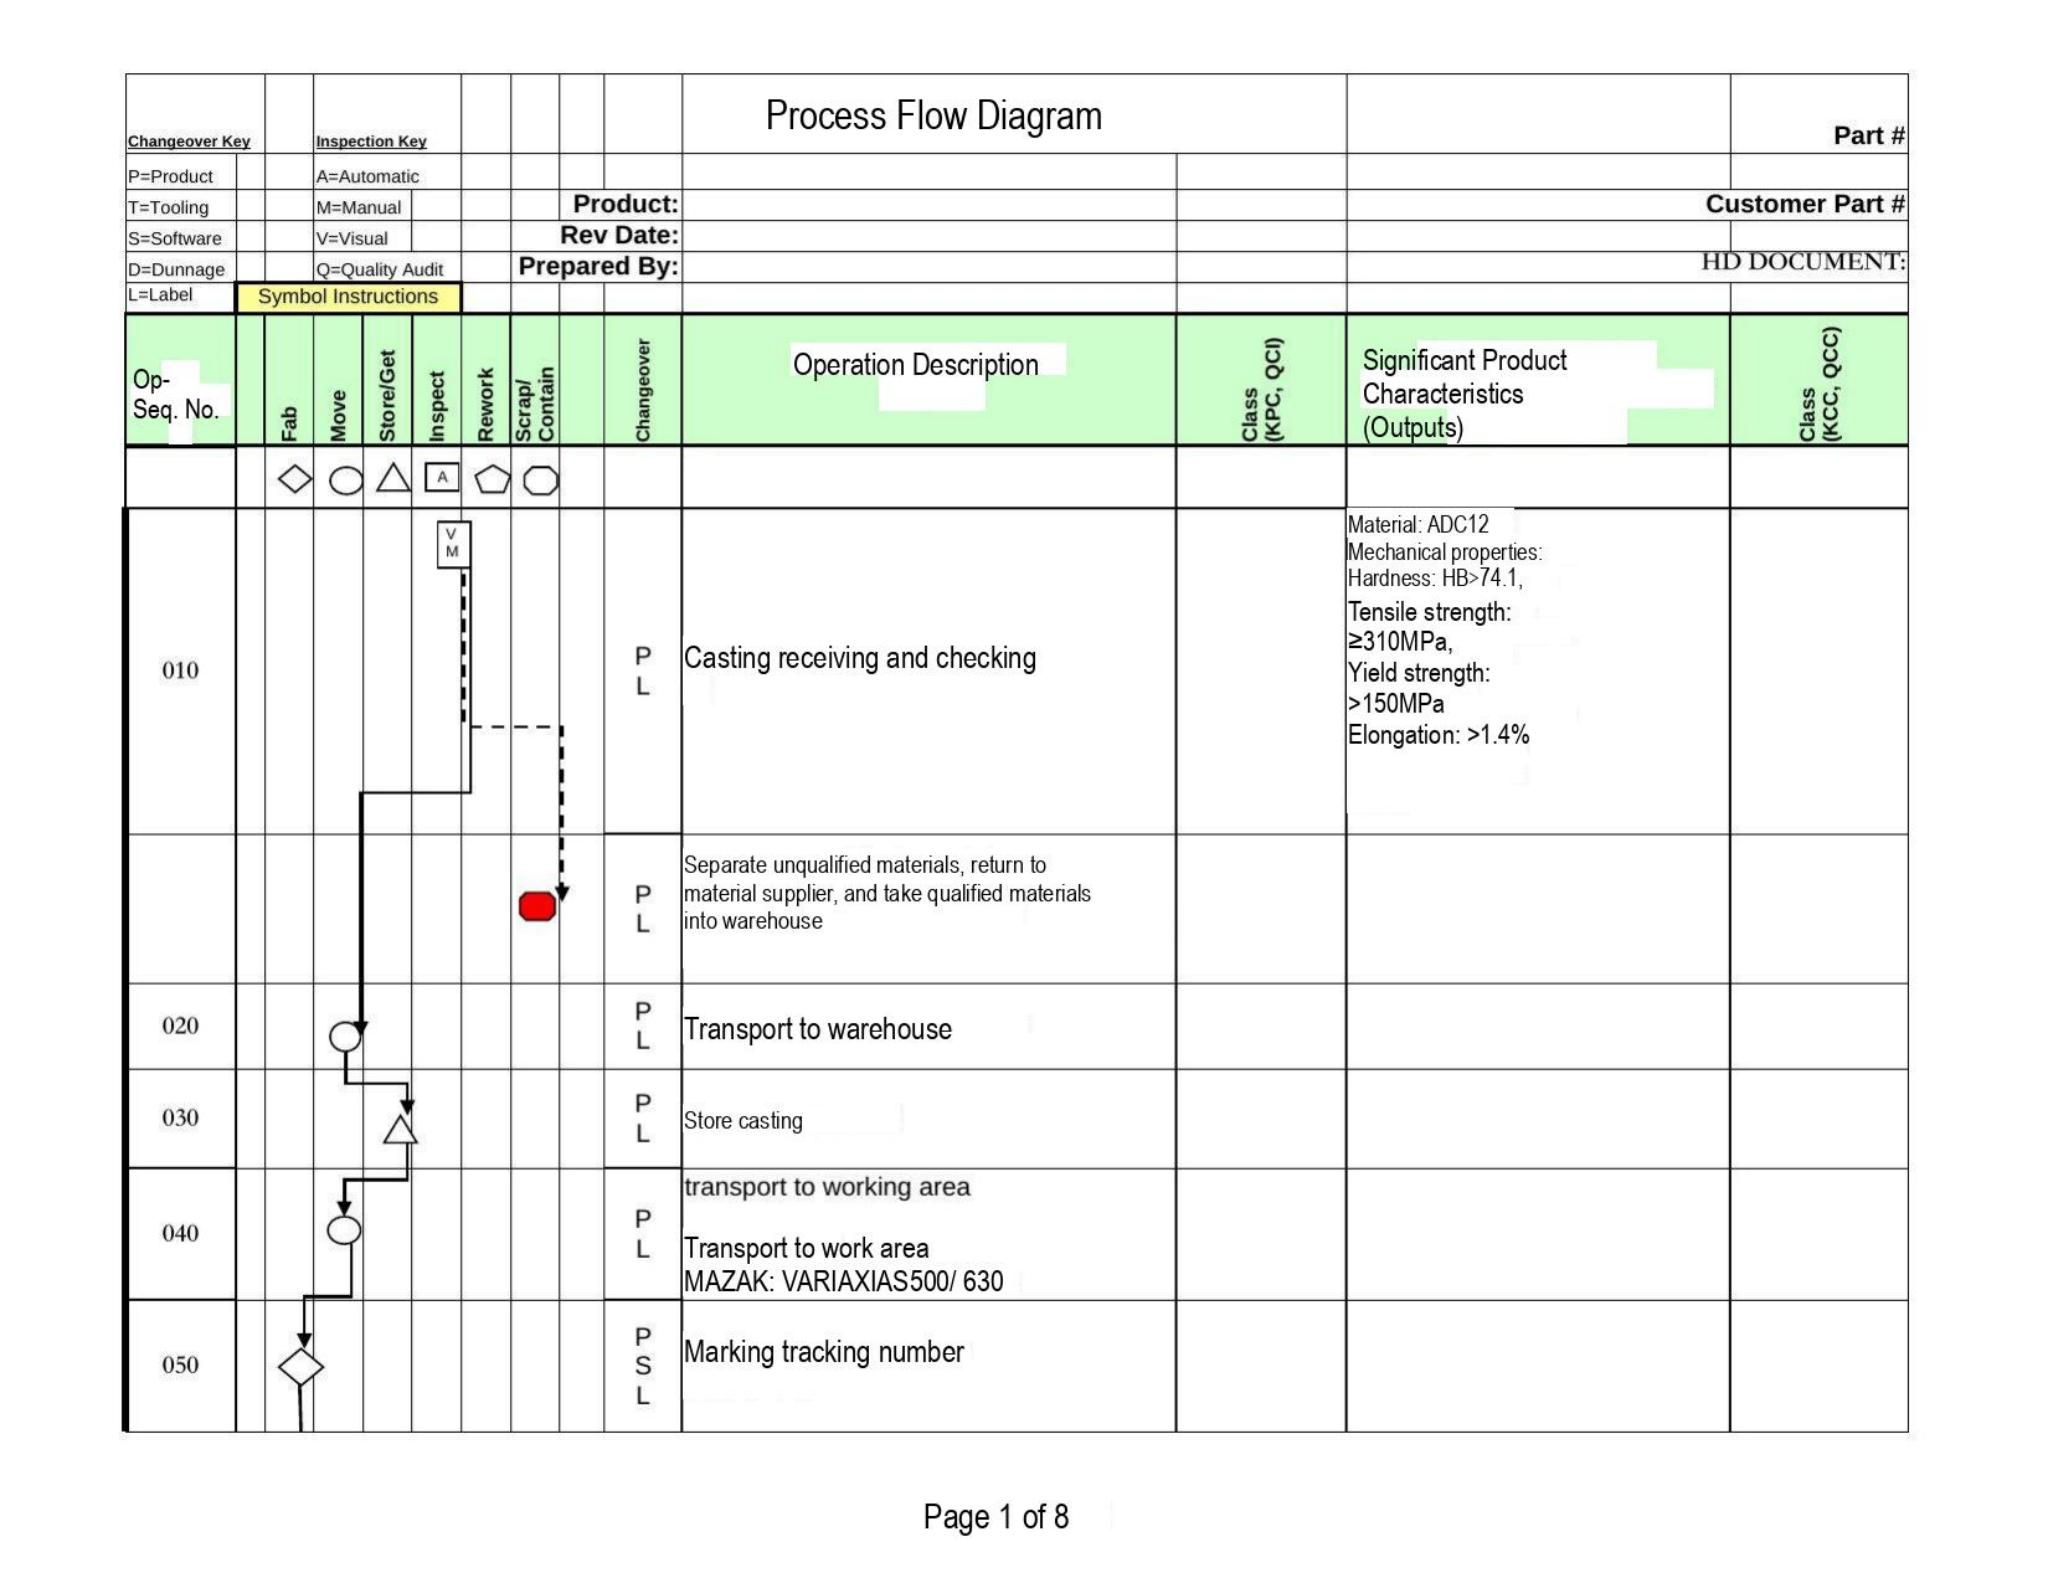Process Flow Diagram

Part #

| Changeover Key | Inspection Key |
|---|---|
| P=Product | A=Automatic |
| T=Tooling | M=Manual |
| S=Software | V=Visual |
| D=Dunnage | Q=Quality Audit |
| L=Label | Symbol Instructions |

Product:
Rev Date:
Prepared By:

Customer Part #
HD DOCUMENT:

| Op-Seq. No. | Fab | Move | Store/Get | Inspect | Rework | Scrap/ Contain | Changeover | Operation Description | Class (KPC, QCI) | Significant Product Characteristics (Outputs) | Class (KCC, QCC) |
|---|---|---|---|---|---|---|---|---|---|---|---|
| | | | | A | | | | | | | |
| 010 | | | | V M | | | P L | Casting receiving and checking | | Material: ADC12 Mechanical properties: Hardness: HB>74.1, Tensile strength: ≥310MPa, Yield strength: >150MPa Elongation: >1.4% | |
| | | | | | | | P L | Separate unqualified materials, return to material supplier, and take qualified materials into warehouse | | | |
| 020 | | | | | | | P L | Transport to warehouse | | | |
| 030 | | | | | | | P L | Store casting | | | |
| 040 | | | | | | | P L | transport to working area<br><br>Transport to work area MAZAK: VARIAXIAS500/ 630 | | | |
| 050 | | | | | | | P S L | Marking tracking number | | | |

Page 1 of 8
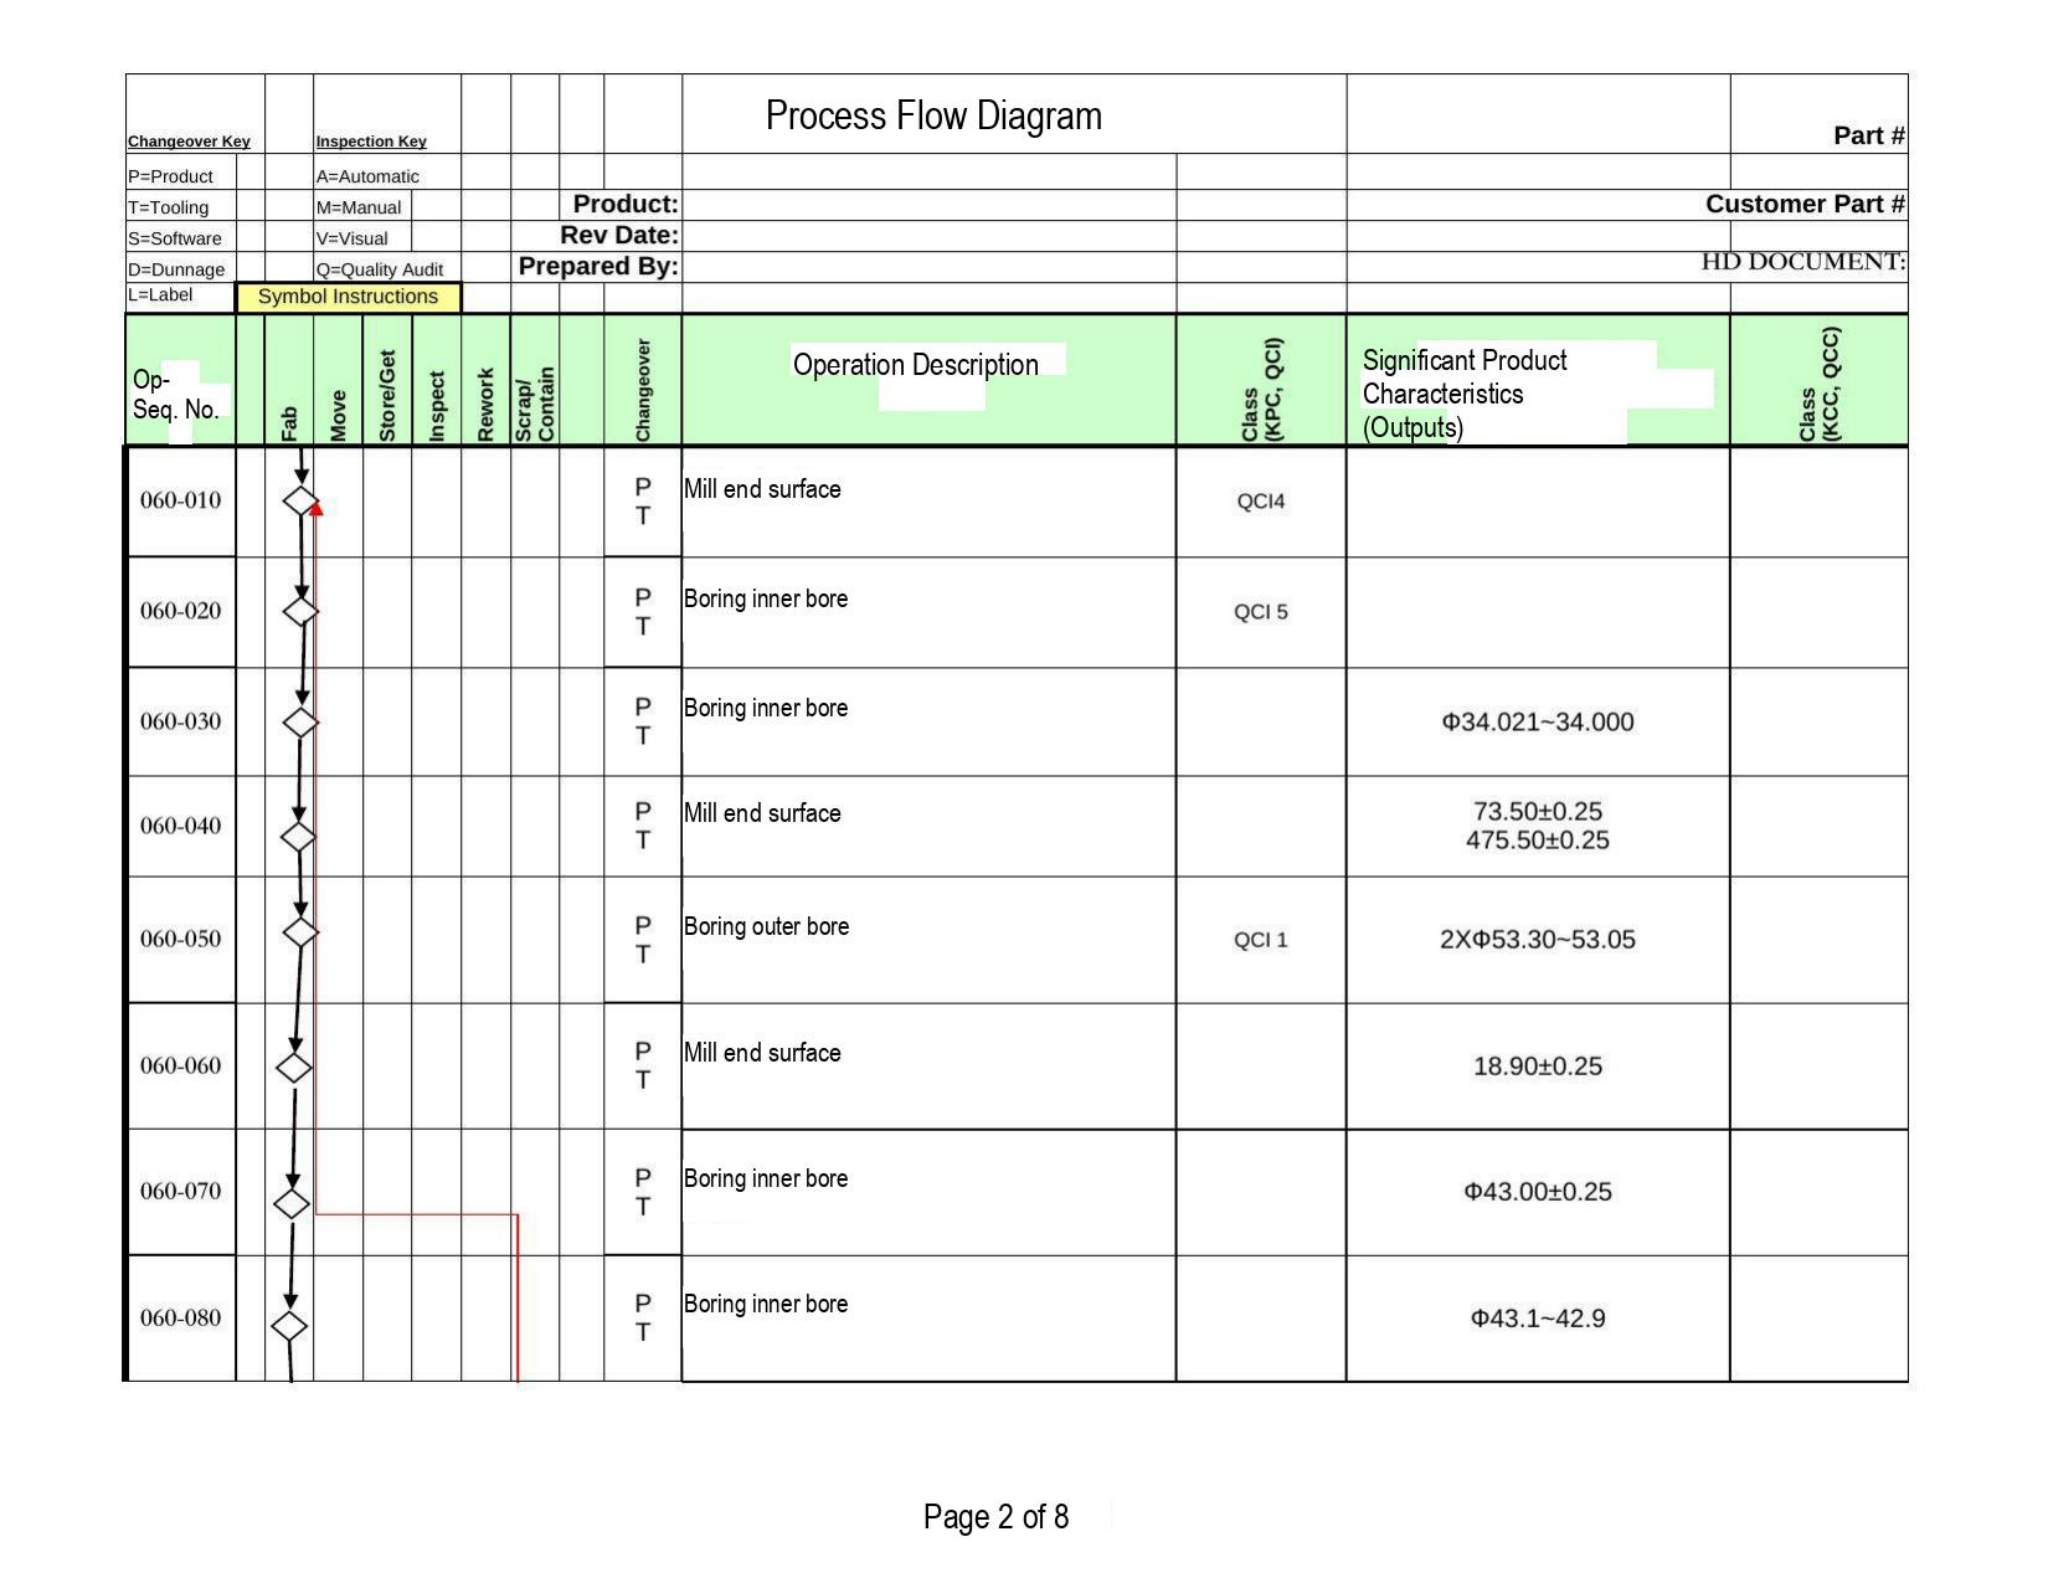Process Flow Diagram

Part #

| Changeover Key | Inspection Key |
|---|---|
| P=Product | A=Automatic |
| T=Tooling | M=Manual |
| S=Software | V=Visual |
| D=Dunnage | Q=Quality Audit |
| L=Label | Symbol Instructions |

Product:
Rev Date:
Prepared By:

Customer Part #
HD DOCUMENT:

| Op-Seq. No. | | Fab | Move | Store/Get | Inspect | Rework | Scrap/Contain | | Changeover | Operation Description | Class (KPC, QCI) | Significant Product Characteristics (Outputs) | Class (KCC, QCC) |
|---|---|---|---|---|---|---|---|---|---|---|---|---|---|
| 060-010 | | | | | | | | | P T | Mill end surface | QCI4 | | |
| 060-020 | | | | | | | | | P T | Boring inner bore | QCI 5 | | |
| 060-030 | | | | | | | | | P T | Boring inner bore | | Φ34.021~34.000 | |
| 060-040 | | | | | | | | | P T | Mill end surface | | 73.50±0.25<br>475.50±0.25 | |
| 060-050 | | | | | | | | | P T | Boring outer bore | QCI 1 | 2XΦ53.30~53.05 | |
| 060-060 | | | | | | | | | P T | Mill end surface | | 18.90±0.25 | |
| 060-070 | | | | | | | | | P T | Boring inner bore | | Φ43.00±0.25 | |
| 060-080 | | | | | | | | | P T | Boring inner bore | | Φ43.1~42.9 | |

Page 2 of 8
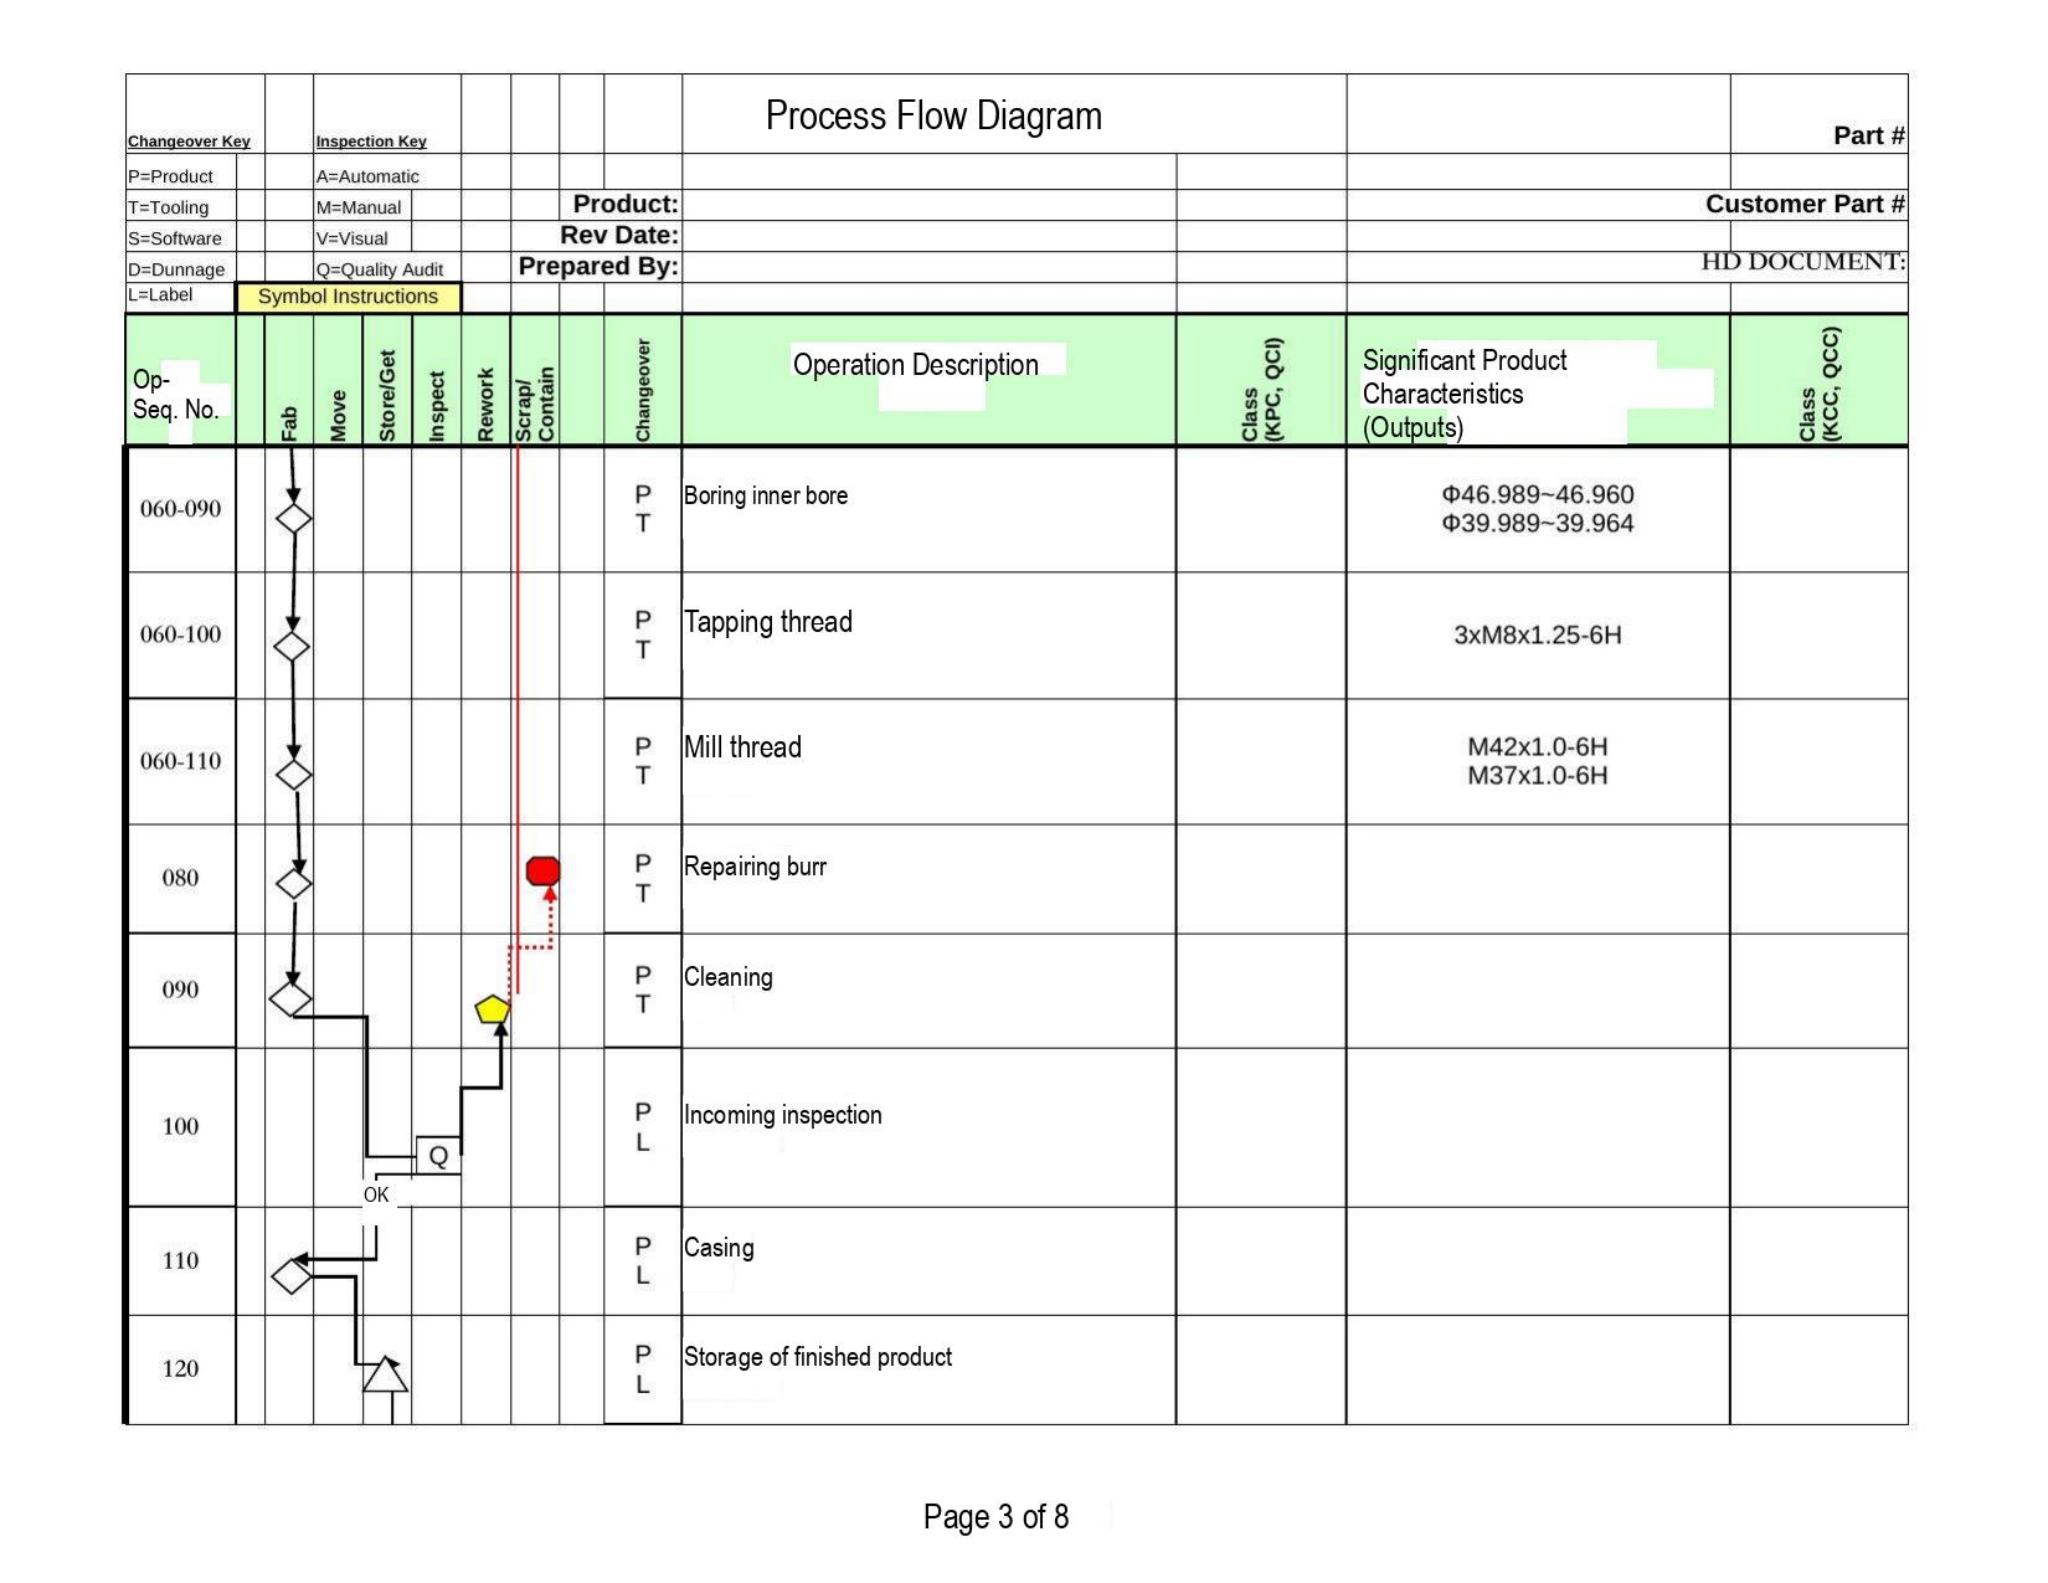Process Flow Diagram

Part #

| Changeover Key | Inspection Key |
|---|---|
| P=Product | A=Automatic |
| T=Tooling | M=Manual |
| S=Software | V=Visual |
| D=Dunnage | Q=Quality Audit |
| L=Label | Symbol Instructions |

Product:
Rev Date:
Prepared By:

Customer Part #
HD DOCUMENT:

| Op-Seq. No. | Fab | Move | Store/Get | Inspect | Rework | Scrap/Contain | Changeover | Operation Description | Class (KPC, QCI) | Significant Product Characteristics (Outputs) | Class (KCC, QCC) |
|---|---|---|---|---|---|---|---|---|---|---|---|
| 060-090 | | | | | | | P T | Boring inner bore | | Φ46.989~46.960 Φ39.989~39.964 | |
| 060-100 | | | | | | | P T | Tapping thread | | 3xM8x1.25-6H | |
| 060-110 | | | | | | | P T | Mill thread | | M42x1.0-6H M37x1.0-6H | |
| 080 | | | | | | | P T | Repairing burr | | | |
| 090 | | | | | | | P T | Cleaning | | | |
| 100 | | | | Q | | | P L | Incoming inspection | | | |
| 110 | | OK | | | | | P L | Casing | | | |
| 120 | | | | | | | P L | Storage of finished product | | | |

Page 3 of 8
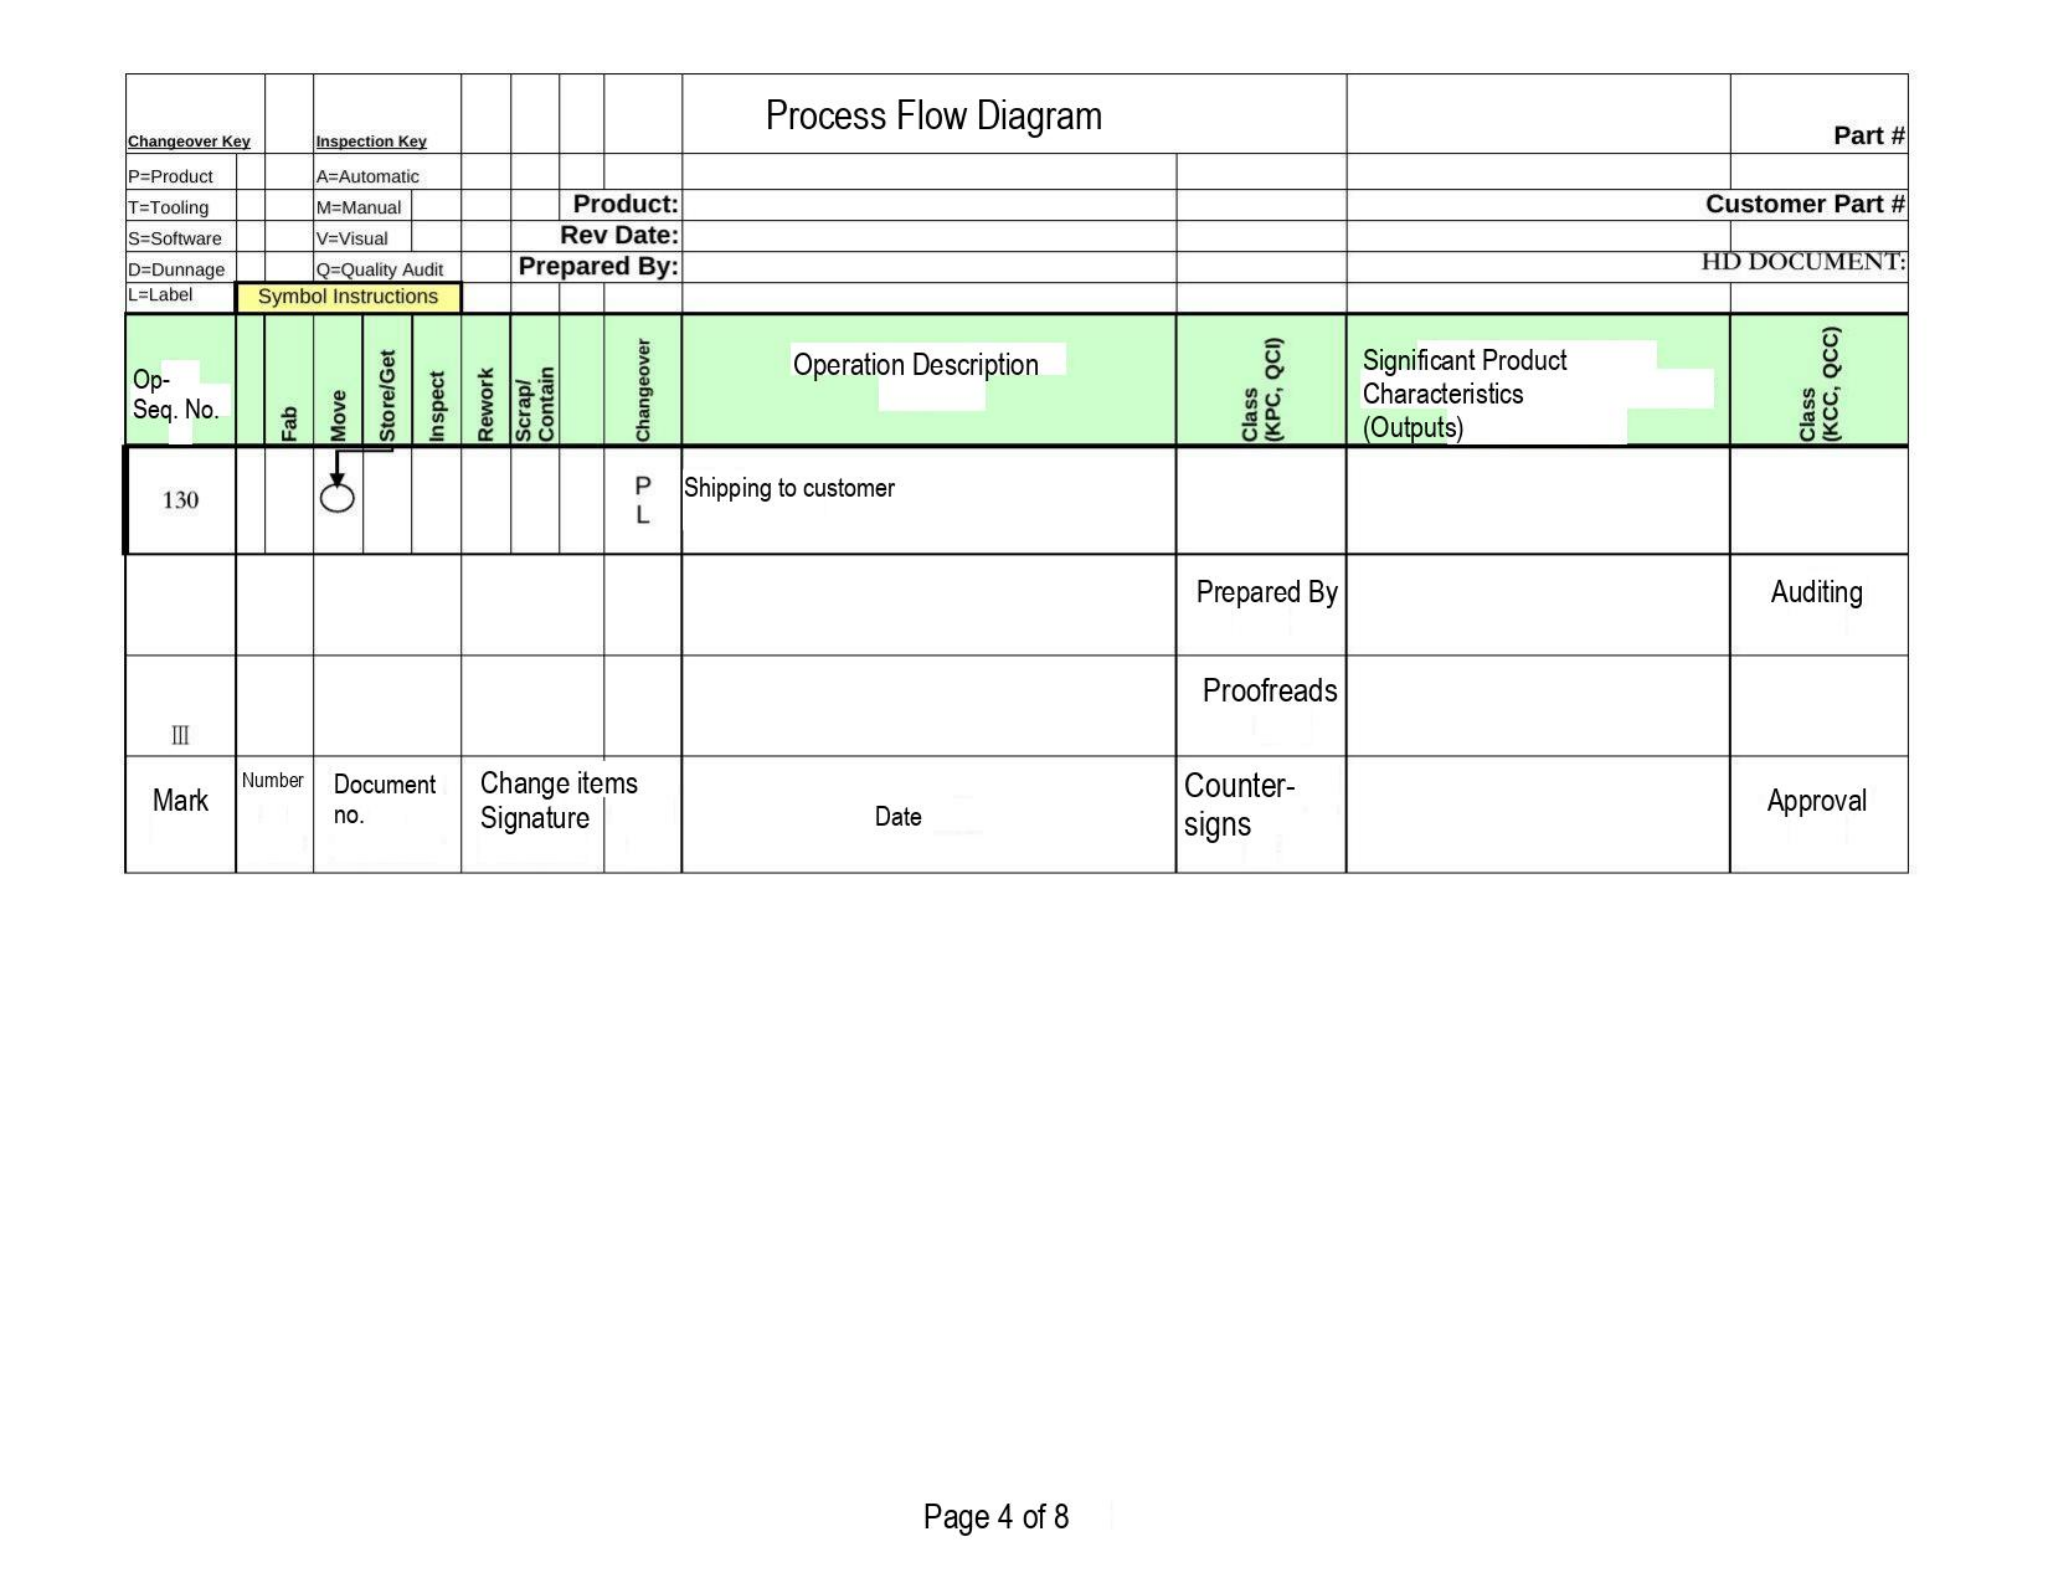Process Flow Diagram

| Changeover Key | Inspection Key | | Part # |
|---|---|---|---|
| P=Product | A=Automatic | | |
| T=Tooling | M=Manual | Product: | Customer Part # |
| S=Software | V=Visual | Rev Date: | |
| D=Dunnage | Q=Quality Audit | Prepared By: | HD DOCUMENT: |
| L=Label | Symbol Instructions | | |

| Op-Seq. No. | Fab | Move | Store/Get | Inspect | Rework | Scrap/ Contain | Changeover | Operation Description | Class (KPC, QCI) | Significant Product Characteristics (Outputs) | Class (KCC, QCC) |
|---|---|---|---|---|---|---|---|---|---|---|---|
| 130 | | | | | | | P L | Shipping to customer | | | |
| | | | | | | | | | Prepared By | | Auditing |
| III | | | | | | | | | Proofreads | | |
| Mark | Number | Document no. | | Change items Signature | | | | Date | Counter-signs | | Approval |

Page 4 of 8
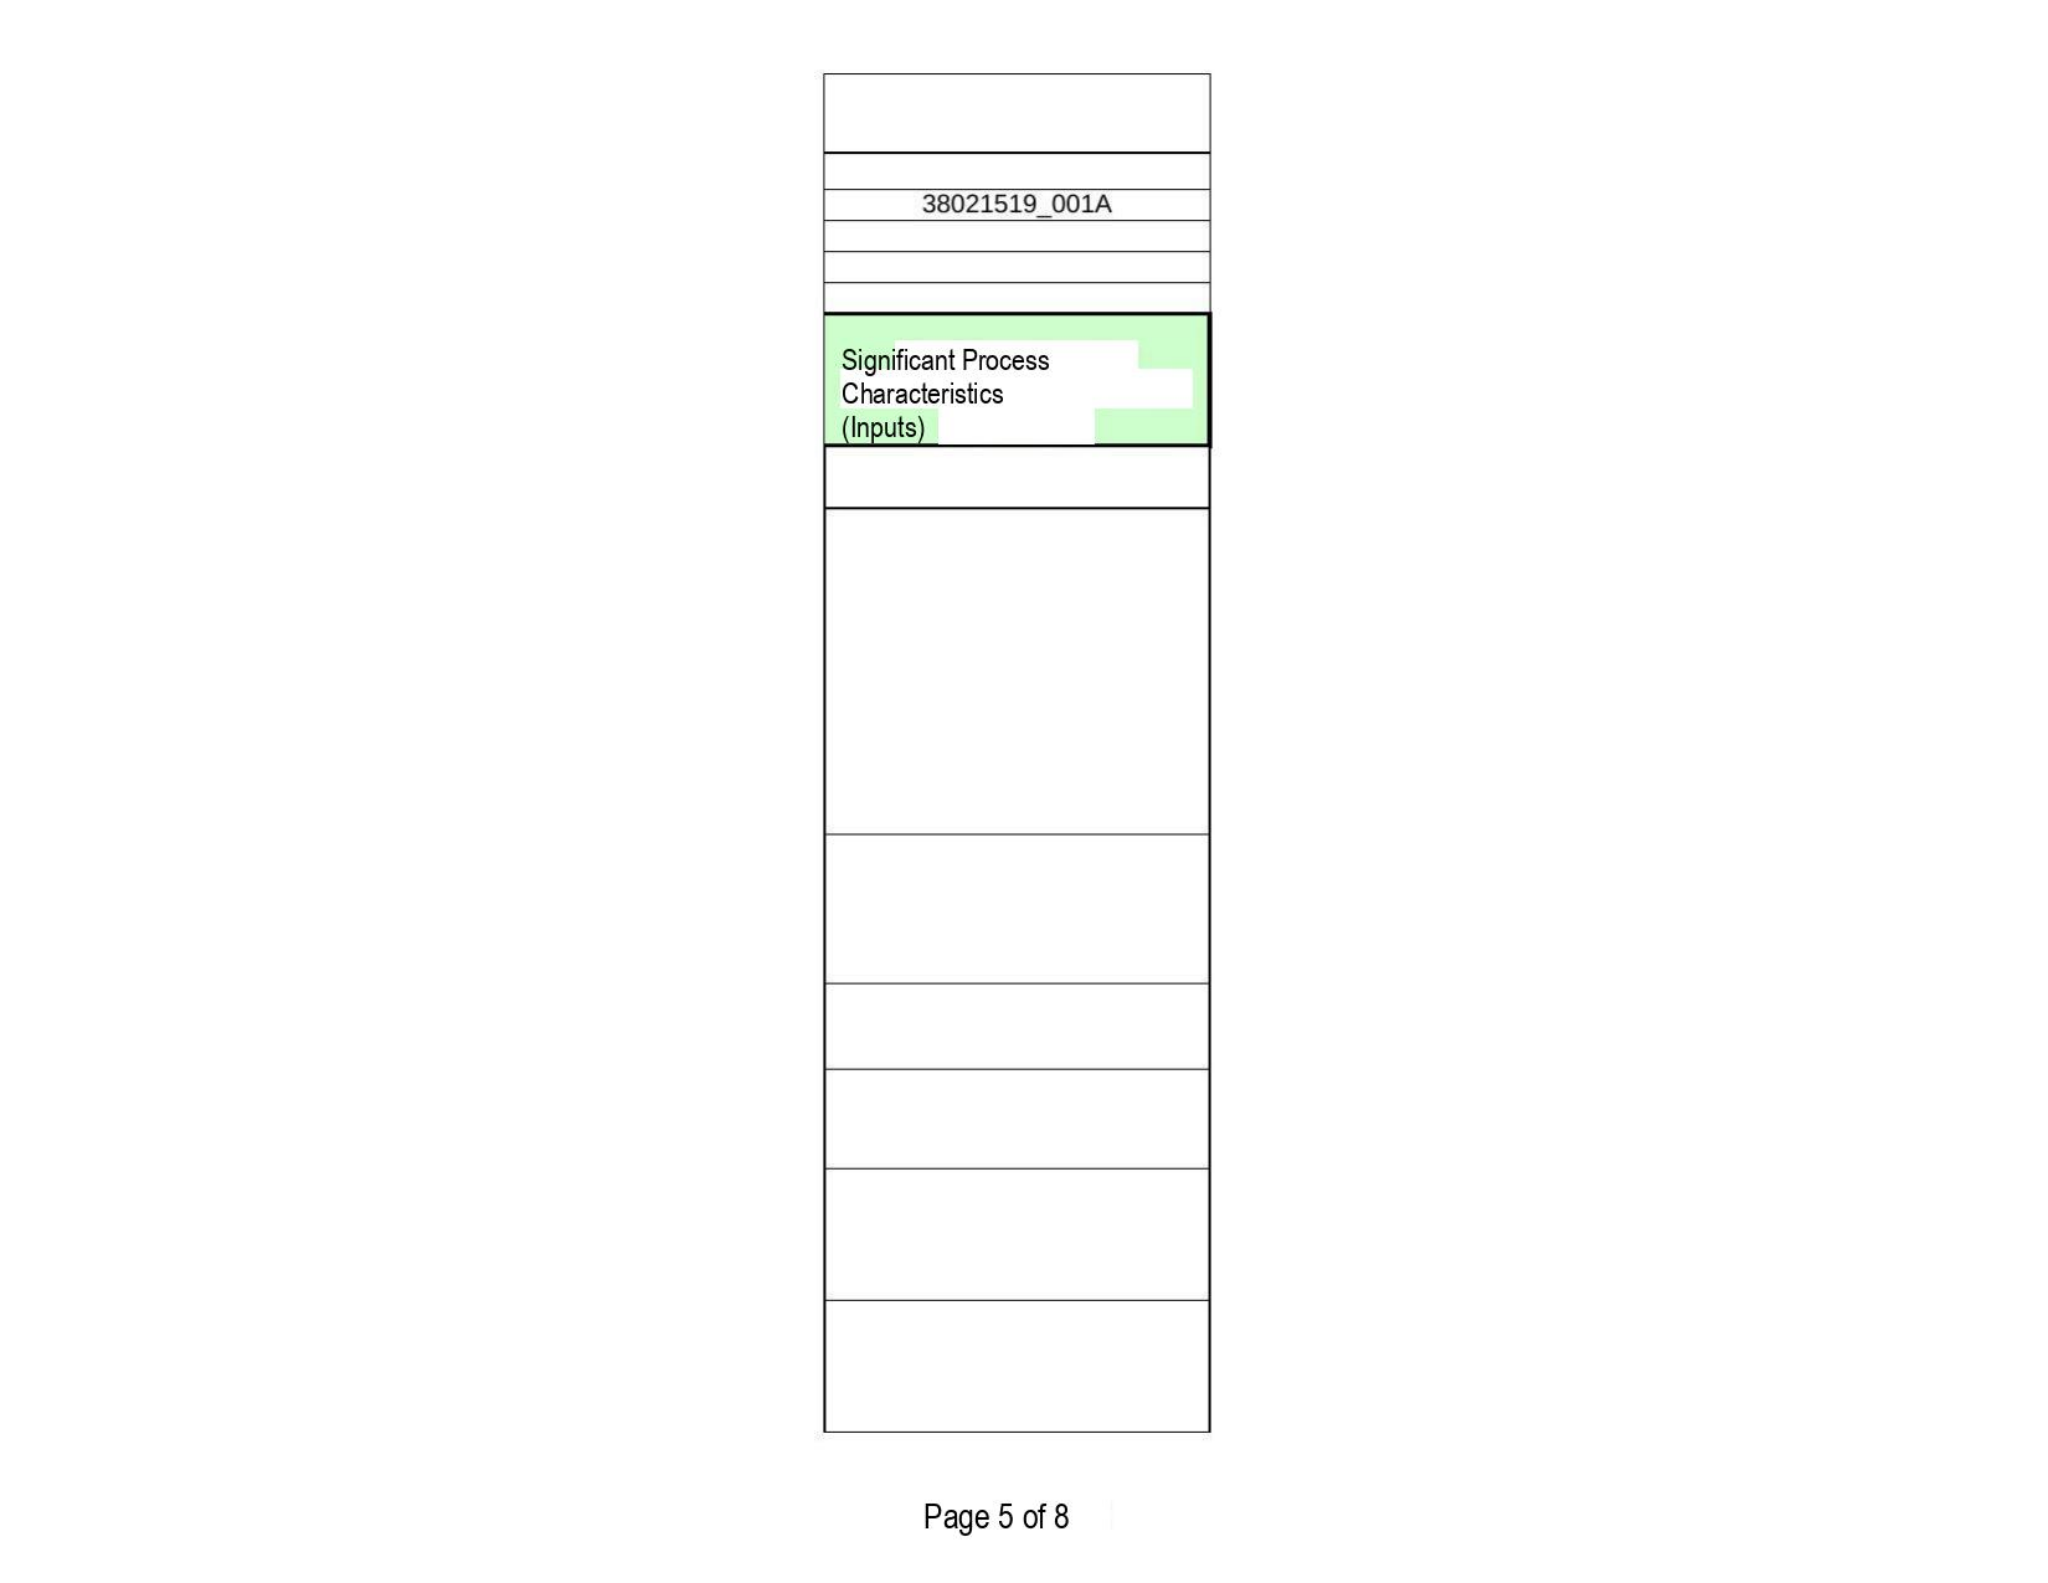| |
|---|
| |
| 38021519_001A |
| |
| |
| |
| Significant Process Characteristics (Inputs) |
| |
| |
| |
| |
| |
| |
| |

Page 5 of 8
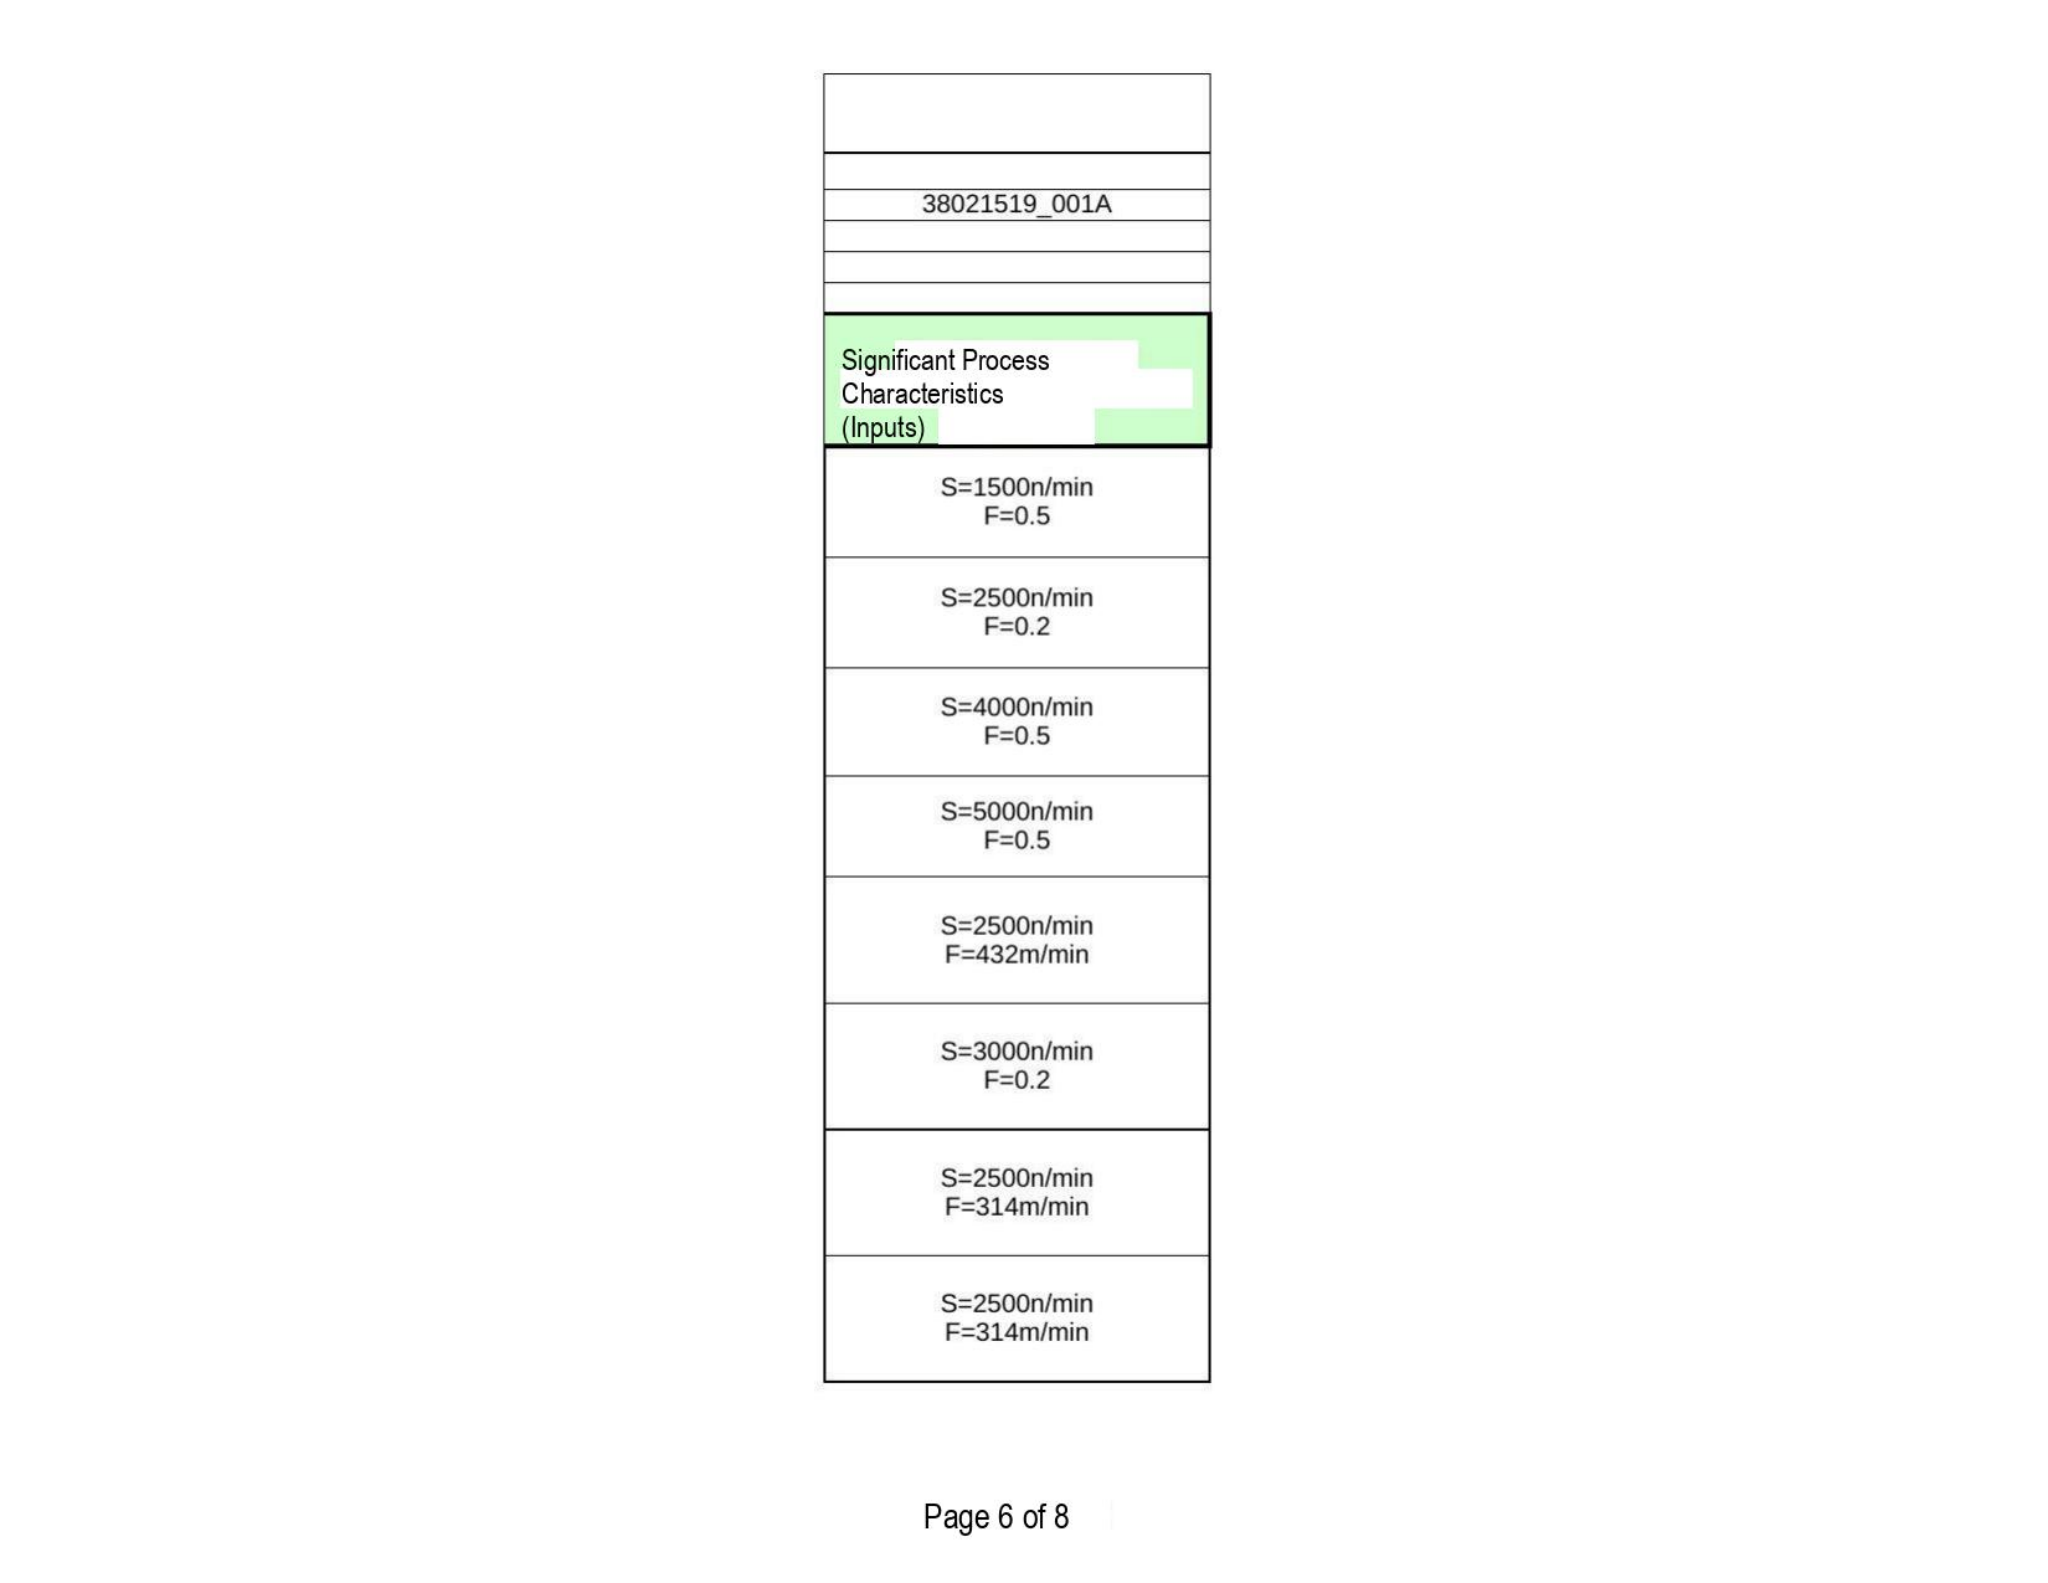38021519_001A

| Significant Process Characteristics (Inputs) |
|---|
| S=1500n/min<br>F=0.5 |
| S=2500n/min<br>F=0.2 |
| S=4000n/min<br>F=0.5 |
| S=5000n/min<br>F=0.5 |
| S=2500n/min<br>F=432m/min |
| S=3000n/min<br>F=0.2 |
| S=2500n/min<br>F=314m/min |
| S=2500n/min<br>F=314m/min |

Page 6 of 8